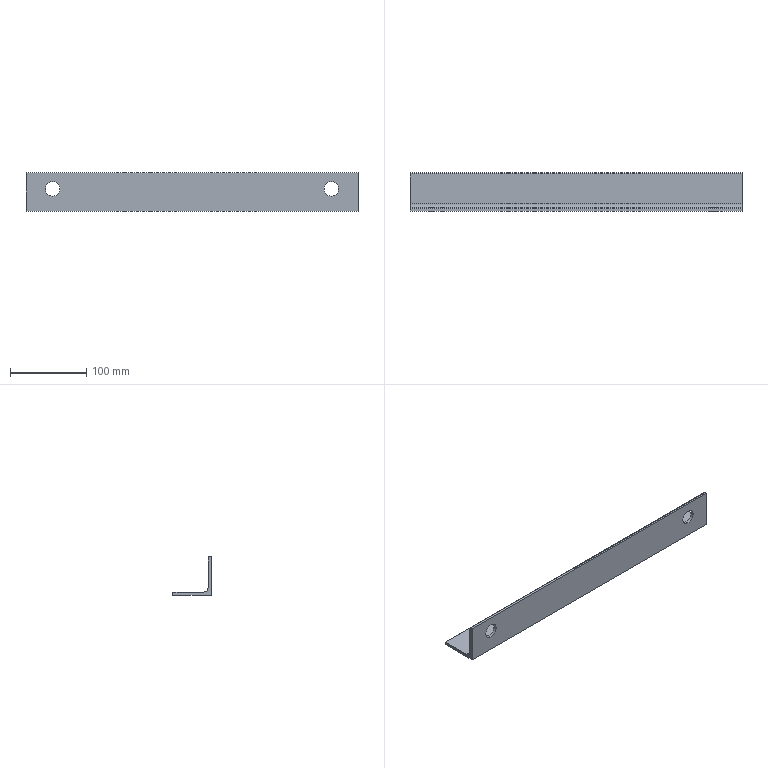Part | STEP file | 电柜楼梯角钢_Default<As Machined> | 1 solid | 15 faces | box 435 x 50 x 50 mm | volume 167265 mm3 | plane 8 | cylinder 7 | commonest cylinder face diameters 19 x4 2.66 x2 11 x1
STEP:
#1=CARTESIAN_POINT('',(0.,0.,0.));
#2=DIRECTION('',(0.,0.,1.));
#3=DIRECTION('',(1.,0.,0.));
#4=AXIS2_PLACEMENT_3D('',#1,#2,#3);
#5=CARTESIAN_POINT('',(-182.5,0.,38.585));
#6=VERTEX_POINT('',#5);
#7=CARTESIAN_POINT('',(-182.5,4.,38.585));
#8=VERTEX_POINT('',#7);
#9=CARTESIAN_POINT('',(-182.5,-6.,38.585));
#10=DIRECTION('',(0.,1.,0.));
#11=VECTOR('',#10,1.);
#12=LINE('',#9,#11);
#13=CARTESIAN_POINT('',(-182.5,-6.,29.085));
#14=DIRECTION('',(0.,1.,0.));
#15=DIRECTION('',(0.,0.,1.));
#16=AXIS2_PLACEMENT_3D('',#13,#14,#15);
#17=CYLINDRICAL_SURFACE('',#16,9.5);
#18=CARTESIAN_POINT('',(6.283,0.));
#19=DIRECTION('',(0.,1.));
#20=VECTOR('',#19,1.);
#21=LINE('',#18,#20);
#22=(GEOMETRIC_REPRESENTATION_CONTEXT(2)PARAMETRIC_REPRESENTATION_CONTEXT()REPRESENTATION_CONTEXT('',''));
#23=DEFINITIONAL_REPRESENTATION('',(#21),#22);
#24=PCURVE('',#17,#23);
#25=CARTESIAN_POINT('',(-182.5,-6.,29.085));
#26=DIRECTION('',(0.,1.,0.));
#27=DIRECTION('',(0.,0.,1.));
#28=AXIS2_PLACEMENT_3D('',#25,#26,#27);
#29=CYLINDRICAL_SURFACE('',#28,9.5);
#30=CARTESIAN_POINT('',(0.,0.));
#31=DIRECTION('',(0.,1.));
#32=VECTOR('',#31,1.);
#33=LINE('',#30,#32);
#34=(GEOMETRIC_REPRESENTATION_CONTEXT(2)PARAMETRIC_REPRESENTATION_CONTEXT()REPRESENTATION_CONTEXT('',''));
#35=DEFINITIONAL_REPRESENTATION('',(#33),#34);
#36=PCURVE('',#29,#35);
#37=SURFACE_CURVE('',#12,(#24,#36),.PCURVE_S1.);
#38=EDGE_CURVE('',#6,#8,#37,.T.);
#39=ORIENTED_EDGE('',*,*,#38,.T.);
#40=CARTESIAN_POINT('',(-182.5,4.,19.585));
#41=VERTEX_POINT('',#40);
#42=CARTESIAN_POINT('',(-182.5,4.,29.085));
#43=DIRECTION('',(0.,1.,0.));
#44=DIRECTION('',(0.,0.,1.));
#45=AXIS2_PLACEMENT_3D('',#42,#43,#44);
#46=CIRCLE('',#45,9.5);
#47=CARTESIAN_POINT('',(0.,10.));
#48=DIRECTION('',(1.,0.));
#49=VECTOR('',#48,1.);
#50=LINE('',#47,#49);
#51=(GEOMETRIC_REPRESENTATION_CONTEXT(2)PARAMETRIC_REPRESENTATION_CONTEXT()REPRESENTATION_CONTEXT('',''));
#52=DEFINITIONAL_REPRESENTATION('',(#50),#51);
#53=PCURVE('',#17,#52);
#54=CARTESIAN_POINT('',(217.5,4.,48.67));
#55=DIRECTION('',(0.,-1.,0.));
#56=DIRECTION('',(1.,0.,0.));
#57=AXIS2_PLACEMENT_3D('',#54,#55,#56);
#58=PLANE('',#57);
#59=CARTESIAN_POINT('',(-400.,-10.085));
#60=CARTESIAN_POINT('',(-383.546,-10.085));
#61=CARTESIAN_POINT('',(-391.773,-24.335));
#62=CARTESIAN_POINT('',(-400.,-38.585));
#63=CARTESIAN_POINT('',(-408.227,-24.335));
#64=CARTESIAN_POINT('',(-416.454,-10.085));
#65=CARTESIAN_POINT('',(-400.,-10.085));
#66=(BOUNDED_CURVE()B_SPLINE_CURVE(2,(#59,#60,#61,#62,#63,#64,#65),.UNSPECIFIED.,.T.,.F.)B_SPLINE_CURVE_WITH_KNOTS((1,2,2,2,2,1),(-2.094,0.,2.094,4.189,6.283,8.378),.UNSPECIFIED.)CURVE()GEOMETRIC_REPRESENTATION_ITEM()RATIONAL_B_SPLINE_CURVE((1.,0.5,1.,0.5,1.,0.5,1.))REPRESENTATION_ITEM(''));
#67=(GEOMETRIC_REPRESENTATION_CONTEXT(2)PARAMETRIC_REPRESENTATION_CONTEXT()REPRESENTATION_CONTEXT('',''));
#68=DEFINITIONAL_REPRESENTATION('',(#66),#67);
#69=PCURVE('',#58,#68);
#70=SURFACE_CURVE('',#46,(#53,#69),.PCURVE_S1.);
#71=EDGE_CURVE('',#41,#8,#70,.T.);
#72=ORIENTED_EDGE('',*,*,#71,.F.);
#73=CARTESIAN_POINT('',(-182.5,0.,19.585));
#74=VERTEX_POINT('',#73);
#75=CARTESIAN_POINT('',(-182.5,-6.,19.585));
#76=DIRECTION('',(0.,1.,0.));
#77=VECTOR('',#76,1.);
#78=LINE('',#75,#77);
#79=CARTESIAN_POINT('',(3.142,0.));
#80=DIRECTION('',(0.,1.));
#81=VECTOR('',#80,1.);
#82=LINE('',#79,#81);
#83=(GEOMETRIC_REPRESENTATION_CONTEXT(2)PARAMETRIC_REPRESENTATION_CONTEXT()REPRESENTATION_CONTEXT('',''));
#84=DEFINITIONAL_REPRESENTATION('',(#82),#83);
#85=PCURVE('',#17,#84);
#86=CARTESIAN_POINT('',(3.142,0.));
#87=DIRECTION('',(0.,1.));
#88=VECTOR('',#87,1.);
#89=LINE('',#86,#88);
#90=(GEOMETRIC_REPRESENTATION_CONTEXT(2)PARAMETRIC_REPRESENTATION_CONTEXT()REPRESENTATION_CONTEXT('',''));
#91=DEFINITIONAL_REPRESENTATION('',(#89),#90);
#92=PCURVE('',#29,#91);
#93=SURFACE_CURVE('',#78,(#85,#92),.PCURVE_S1.);
#94=EDGE_CURVE('',#74,#41,#93,.T.);
#95=ORIENTED_EDGE('',*,*,#94,.F.);
#96=CARTESIAN_POINT('',(-182.5,0.,29.085));
#97=DIRECTION('',(0.,1.,0.));
#98=DIRECTION('',(-1.,0.,0.));
#99=AXIS2_PLACEMENT_3D('',#96,#97,#98);
#100=CIRCLE('',#99,9.5);
#101=CARTESIAN_POINT('',(-1.571,6.));
#102=DIRECTION('',(1.,0.));
#103=VECTOR('',#102,1.);
#104=LINE('',#101,#103);
#105=(GEOMETRIC_REPRESENTATION_CONTEXT(2)PARAMETRIC_REPRESENTATION_CONTEXT()REPRESENTATION_CONTEXT('',''));
#106=DEFINITIONAL_REPRESENTATION('',(#104),#105);
#107=PCURVE('',#17,#106);
#108=CARTESIAN_POINT('',(217.5,0.,50.));
#109=DIRECTION('',(0.,1.,0.));
#110=DIRECTION('',(-1.,0.,0.));
#111=AXIS2_PLACEMENT_3D('',#108,#109,#110);
#112=PLANE('',#111);
#113=CARTESIAN_POINT('',(400.,-20.915));
#114=DIRECTION('',(1.,0.));
#115=AXIS2_PLACEMENT_2D('',#113,#114);
#116=CIRCLE('',#115,9.5);
#117=(GEOMETRIC_REPRESENTATION_CONTEXT(2)PARAMETRIC_REPRESENTATION_CONTEXT()REPRESENTATION_CONTEXT('',''));
#118=DEFINITIONAL_REPRESENTATION('',(#116),#117);
#119=PCURVE('',#112,#118);
#120=SURFACE_CURVE('',#100,(#107,#119),.PCURVE_S1.);
#121=EDGE_CURVE('',#74,#6,#120,.T.);
#122=ORIENTED_EDGE('',*,*,#121,.T.);
#123=EDGE_LOOP('',(#39,#72,#95,#122));
#124=FACE_BOUND('',#123,.F.);
#125=ADVANCED_FACE('',(#124),#17,.F.);
#126=CARTESIAN_POINT('',(182.5,0.,38.585));
#127=VERTEX_POINT('',#126);
#128=CARTESIAN_POINT('',(182.5,4.,38.585));
#129=VERTEX_POINT('',#128);
#130=CARTESIAN_POINT('',(182.5,-6.,38.585));
#131=DIRECTION('',(0.,1.,0.));
#132=VECTOR('',#131,1.);
#133=LINE('',#130,#132);
#134=CARTESIAN_POINT('',(182.5,-6.,29.085));
#135=DIRECTION('',(0.,1.,0.));
#136=DIRECTION('',(0.,0.,1.));
#137=AXIS2_PLACEMENT_3D('',#134,#135,#136);
#138=CYLINDRICAL_SURFACE('',#137,9.5);
#139=CARTESIAN_POINT('',(6.283,0.));
#140=DIRECTION('',(0.,1.));
#141=VECTOR('',#140,1.);
#142=LINE('',#139,#141);
#143=(GEOMETRIC_REPRESENTATION_CONTEXT(2)PARAMETRIC_REPRESENTATION_CONTEXT()REPRESENTATION_CONTEXT('',''));
#144=DEFINITIONAL_REPRESENTATION('',(#142),#143);
#145=PCURVE('',#138,#144);
#146=CARTESIAN_POINT('',(182.5,-6.,29.085));
#147=DIRECTION('',(0.,1.,0.));
#148=DIRECTION('',(0.,0.,1.));
#149=AXIS2_PLACEMENT_3D('',#146,#147,#148);
#150=CYLINDRICAL_SURFACE('',#149,9.5);
#151=CARTESIAN_POINT('',(0.,0.));
#152=DIRECTION('',(0.,1.));
#153=VECTOR('',#152,1.);
#154=LINE('',#151,#153);
#155=(GEOMETRIC_REPRESENTATION_CONTEXT(2)PARAMETRIC_REPRESENTATION_CONTEXT()REPRESENTATION_CONTEXT('',''));
#156=DEFINITIONAL_REPRESENTATION('',(#154),#155);
#157=PCURVE('',#150,#156);
#158=SURFACE_CURVE('',#133,(#145,#157),.PCURVE_S1.);
#159=EDGE_CURVE('',#127,#129,#158,.T.);
#160=ORIENTED_EDGE('',*,*,#159,.T.);
#161=CARTESIAN_POINT('',(182.5,4.,19.585));
#162=VERTEX_POINT('',#161);
#163=CARTESIAN_POINT('',(182.5,4.,29.085));
#164=DIRECTION('',(0.,1.,0.));
#165=DIRECTION('',(0.,0.,-1.));
#166=AXIS2_PLACEMENT_3D('',#163,#164,#165);
#167=CIRCLE('',#166,9.5);
#168=CARTESIAN_POINT('',(3.142,10.));
#169=DIRECTION('',(1.,0.));
#170=VECTOR('',#169,1.);
#171=LINE('',#168,#170);
#172=(GEOMETRIC_REPRESENTATION_CONTEXT(2)PARAMETRIC_REPRESENTATION_CONTEXT()REPRESENTATION_CONTEXT('',''));
#173=DEFINITIONAL_REPRESENTATION('',(#171),#172);
#174=PCURVE('',#138,#173);
#175=CARTESIAN_POINT('',(-35.,-29.085));
#176=CARTESIAN_POINT('',(-51.454,-29.085));
#177=CARTESIAN_POINT('',(-43.227,-14.835));
#178=CARTESIAN_POINT('',(-35.,-0.585));
#179=CARTESIAN_POINT('',(-26.773,-14.835));
#180=CARTESIAN_POINT('',(-18.546,-29.085));
#181=CARTESIAN_POINT('',(-35.,-29.085));
#182=(BOUNDED_CURVE()B_SPLINE_CURVE(2,(#175,#176,#177,#178,#179,#180,#181),.UNSPECIFIED.,.T.,.F.)B_SPLINE_CURVE_WITH_KNOTS((1,2,2,2,2,1),(-2.094,0.,2.094,4.189,6.283,8.378),.UNSPECIFIED.)CURVE()GEOMETRIC_REPRESENTATION_ITEM()RATIONAL_B_SPLINE_CURVE((1.,0.5,1.,0.5,1.,0.5,1.))REPRESENTATION_ITEM(''));
#183=(GEOMETRIC_REPRESENTATION_CONTEXT(2)PARAMETRIC_REPRESENTATION_CONTEXT()REPRESENTATION_CONTEXT('',''));
#184=DEFINITIONAL_REPRESENTATION('',(#182),#183);
#185=PCURVE('',#58,#184);
#186=SURFACE_CURVE('',#167,(#174,#185),.PCURVE_S1.);
#187=EDGE_CURVE('',#162,#129,#186,.T.);
#188=ORIENTED_EDGE('',*,*,#187,.F.);
#189=CARTESIAN_POINT('',(182.5,0.,19.585));
#190=VERTEX_POINT('',#189);
#191=CARTESIAN_POINT('',(182.5,-6.,19.585));
#192=DIRECTION('',(0.,1.,0.));
#193=VECTOR('',#192,1.);
#194=LINE('',#191,#193);
#195=CARTESIAN_POINT('',(3.142,0.));
#196=DIRECTION('',(0.,1.));
#197=VECTOR('',#196,1.);
#198=LINE('',#195,#197);
#199=(GEOMETRIC_REPRESENTATION_CONTEXT(2)PARAMETRIC_REPRESENTATION_CONTEXT()REPRESENTATION_CONTEXT('',''));
#200=DEFINITIONAL_REPRESENTATION('',(#198),#199);
#201=PCURVE('',#138,#200);
#202=CARTESIAN_POINT('',(3.142,0.));
#203=DIRECTION('',(0.,1.));
#204=VECTOR('',#203,1.);
#205=LINE('',#202,#204);
#206=(GEOMETRIC_REPRESENTATION_CONTEXT(2)PARAMETRIC_REPRESENTATION_CONTEXT()REPRESENTATION_CONTEXT('',''));
#207=DEFINITIONAL_REPRESENTATION('',(#205),#206);
#208=PCURVE('',#150,#207);
#209=SURFACE_CURVE('',#194,(#201,#208),.PCURVE_S1.);
#210=EDGE_CURVE('',#190,#162,#209,.T.);
#211=ORIENTED_EDGE('',*,*,#210,.F.);
#212=CARTESIAN_POINT('',(182.5,0.,29.085));
#213=DIRECTION('',(0.,1.,0.));
#214=DIRECTION('',(-1.,0.,0.));
#215=AXIS2_PLACEMENT_3D('',#212,#213,#214);
#216=CIRCLE('',#215,9.5);
#217=CARTESIAN_POINT('',(-1.571,6.));
#218=DIRECTION('',(1.,0.));
#219=VECTOR('',#218,1.);
#220=LINE('',#217,#219);
#221=(GEOMETRIC_REPRESENTATION_CONTEXT(2)PARAMETRIC_REPRESENTATION_CONTEXT()REPRESENTATION_CONTEXT('',''));
#222=DEFINITIONAL_REPRESENTATION('',(#220),#221);
#223=PCURVE('',#138,#222);
#224=CARTESIAN_POINT('',(35.,-20.915));
#225=DIRECTION('',(1.,0.));
#226=AXIS2_PLACEMENT_2D('',#224,#225);
#227=CIRCLE('',#226,9.5);
#228=(GEOMETRIC_REPRESENTATION_CONTEXT(2)PARAMETRIC_REPRESENTATION_CONTEXT()REPRESENTATION_CONTEXT('',''));
#229=DEFINITIONAL_REPRESENTATION('',(#227),#228);
#230=PCURVE('',#112,#229);
#231=SURFACE_CURVE('',#216,(#223,#230),.PCURVE_S1.);
#232=EDGE_CURVE('',#190,#127,#231,.T.);
#233=ORIENTED_EDGE('',*,*,#232,.T.);
#234=EDGE_LOOP('',(#160,#188,#211,#233));
#235=FACE_BOUND('',#234,.F.);
#236=ADVANCED_FACE('',(#235),#138,.F.);
#237=CARTESIAN_POINT('',(-217.5,50.,2.67));
#238=VERTEX_POINT('',#237);
#239=CARTESIAN_POINT('',(-217.5,48.67,4.));
#240=VERTEX_POINT('',#239);
#241=CARTESIAN_POINT('',(-217.5,48.67,2.67));
#242=DIRECTION('',(1.,0.,0.));
#243=DIRECTION('',(0.,1.,0.));
#244=AXIS2_PLACEMENT_3D('',#241,#242,#243);
#245=CIRCLE('',#244,1.33);
#246=CARTESIAN_POINT('',(217.5,48.67,2.67));
#247=DIRECTION('',(-1.,0.,0.));
#248=DIRECTION('',(0.,-1.,0.));
#249=AXIS2_PLACEMENT_3D('',#246,#247,#248);
#250=CYLINDRICAL_SURFACE('',#249,1.33);
#251=CARTESIAN_POINT('',(3.142,435.));
#252=DIRECTION('',(-1.,0.));
#253=VECTOR('',#252,1.);
#254=LINE('',#251,#253);
#255=(GEOMETRIC_REPRESENTATION_CONTEXT(2)PARAMETRIC_REPRESENTATION_CONTEXT()REPRESENTATION_CONTEXT('',''));
#256=DEFINITIONAL_REPRESENTATION('',(#254),#255);
#257=PCURVE('',#250,#256);
#258=CARTESIAN_POINT('',(-217.5,48.67,2.67));
#259=DIRECTION('',(1.,0.,0.));
#260=DIRECTION('',(0.,1.,0.));
#261=AXIS2_PLACEMENT_3D('',#258,#259,#260);
#262=PLANE('',#261);
#263=CARTESIAN_POINT('',(0.,0.));
#264=DIRECTION('',(1.,0.));
#265=AXIS2_PLACEMENT_2D('',#263,#264);
#266=CIRCLE('',#265,1.33);
#267=(GEOMETRIC_REPRESENTATION_CONTEXT(2)PARAMETRIC_REPRESENTATION_CONTEXT()REPRESENTATION_CONTEXT('',''));
#268=DEFINITIONAL_REPRESENTATION('',(#266),#267);
#269=PCURVE('',#262,#268);
#270=SURFACE_CURVE('',#245,(#257,#269),.PCURVE_S1.);
#271=EDGE_CURVE('',#238,#240,#270,.T.);
#272=ORIENTED_EDGE('',*,*,#271,.T.);
#273=CARTESIAN_POINT('',(217.5,48.67,4.));
#274=VERTEX_POINT('',#273);
#275=CARTESIAN_POINT('',(217.5,48.67,4.));
#276=DIRECTION('',(-1.,0.,0.));
#277=VECTOR('',#276,1.);
#278=LINE('',#275,#277);
#279=CARTESIAN_POINT('',(1.571,0.));
#280=DIRECTION('',(0.,1.));
#281=VECTOR('',#280,1.);
#282=LINE('',#279,#281);
#283=(GEOMETRIC_REPRESENTATION_CONTEXT(2)PARAMETRIC_REPRESENTATION_CONTEXT()REPRESENTATION_CONTEXT('',''));
#284=DEFINITIONAL_REPRESENTATION('',(#282),#283);
#285=PCURVE('',#250,#284);
#286=CARTESIAN_POINT('',(217.5,9.5,4.));
#287=DIRECTION('',(0.,0.,-1.));
#288=DIRECTION('',(-1.,0.,0.));
#289=AXIS2_PLACEMENT_3D('',#286,#287,#288);
#290=PLANE('',#289);
#291=CARTESIAN_POINT('',(0.,39.17));
#292=DIRECTION('',(1.,0.));
#293=VECTOR('',#292,1.);
#294=LINE('',#291,#293);
#295=(GEOMETRIC_REPRESENTATION_CONTEXT(2)PARAMETRIC_REPRESENTATION_CONTEXT()REPRESENTATION_CONTEXT('',''));
#296=DEFINITIONAL_REPRESENTATION('',(#294),#295);
#297=PCURVE('',#290,#296);
#298=SURFACE_CURVE('',#278,(#285,#297),.PCURVE_S1.);
#299=EDGE_CURVE('',#274,#240,#298,.T.);
#300=ORIENTED_EDGE('',*,*,#299,.F.);
#301=CARTESIAN_POINT('',(217.5,50.,2.67));
#302=VERTEX_POINT('',#301);
#303=CARTESIAN_POINT('',(217.5,48.67,2.67));
#304=DIRECTION('',(1.,0.,0.));
#305=DIRECTION('',(0.,1.,0.));
#306=AXIS2_PLACEMENT_3D('',#303,#304,#305);
#307=CIRCLE('',#306,1.33);
#308=CARTESIAN_POINT('',(3.142,0.));
#309=DIRECTION('',(-1.,0.));
#310=VECTOR('',#309,1.);
#311=LINE('',#308,#310);
#312=(GEOMETRIC_REPRESENTATION_CONTEXT(2)PARAMETRIC_REPRESENTATION_CONTEXT()REPRESENTATION_CONTEXT('',''));
#313=DEFINITIONAL_REPRESENTATION('',(#311),#312);
#314=PCURVE('',#250,#313);
#315=CARTESIAN_POINT('',(217.5,48.67,2.67));
#316=DIRECTION('',(1.,0.,0.));
#317=DIRECTION('',(0.,1.,0.));
#318=AXIS2_PLACEMENT_3D('',#315,#316,#317);
#319=PLANE('',#318);
#320=CARTESIAN_POINT('',(0.,0.));
#321=DIRECTION('',(1.,0.));
#322=AXIS2_PLACEMENT_2D('',#320,#321);
#323=CIRCLE('',#322,1.33);
#324=(GEOMETRIC_REPRESENTATION_CONTEXT(2)PARAMETRIC_REPRESENTATION_CONTEXT()REPRESENTATION_CONTEXT('',''));
#325=DEFINITIONAL_REPRESENTATION('',(#323),#324);
#326=PCURVE('',#319,#325);
#327=SURFACE_CURVE('',#307,(#314,#326),.PCURVE_S1.);
#328=EDGE_CURVE('',#302,#274,#327,.T.);
#329=ORIENTED_EDGE('',*,*,#328,.F.);
#330=CARTESIAN_POINT('',(217.5,50.,2.67));
#331=DIRECTION('',(-1.,0.,0.));
#332=VECTOR('',#331,1.);
#333=LINE('',#330,#332);
#334=CARTESIAN_POINT('',(3.142,0.));
#335=DIRECTION('',(0.,1.));
#336=VECTOR('',#335,1.);
#337=LINE('',#334,#336);
#338=(GEOMETRIC_REPRESENTATION_CONTEXT(2)PARAMETRIC_REPRESENTATION_CONTEXT()REPRESENTATION_CONTEXT('',''));
#339=DEFINITIONAL_REPRESENTATION('',(#337),#338);
#340=PCURVE('',#250,#339);
#341=CARTESIAN_POINT('',(217.5,50.,2.67));
#342=DIRECTION('',(0.,-1.,0.));
#343=DIRECTION('',(1.,0.,0.));
#344=AXIS2_PLACEMENT_3D('',#341,#342,#343);
#345=PLANE('',#344);
#346=CARTESIAN_POINT('',(0.,0.));
#347=DIRECTION('',(-1.,0.));
#348=VECTOR('',#347,1.);
#349=LINE('',#346,#348);
#350=(GEOMETRIC_REPRESENTATION_CONTEXT(2)PARAMETRIC_REPRESENTATION_CONTEXT()REPRESENTATION_CONTEXT('',''));
#351=DEFINITIONAL_REPRESENTATION('',(#349),#350);
#352=PCURVE('',#345,#351);
#353=SURFACE_CURVE('',#333,(#340,#352),.PCURVE_S1.);
#354=EDGE_CURVE('',#302,#238,#353,.T.);
#355=ORIENTED_EDGE('',*,*,#354,.T.);
#356=EDGE_LOOP('',(#272,#300,#329,#355));
#357=FACE_BOUND('',#356,.T.);
#358=ADVANCED_FACE('',(#357),#250,.T.);
#359=CARTESIAN_POINT('',(-217.5,9.5,4.));
#360=VERTEX_POINT('',#359);
#361=CARTESIAN_POINT('',(-217.5,9.5,4.));
#362=DIRECTION('',(0.,-1.,0.));
#363=VECTOR('',#362,1.);
#364=LINE('',#361,#363);
#365=CARTESIAN_POINT('',(435.,0.));
#366=DIRECTION('',(0.,-1.));
#367=VECTOR('',#366,1.);
#368=LINE('',#365,#367);
#369=(GEOMETRIC_REPRESENTATION_CONTEXT(2)PARAMETRIC_REPRESENTATION_CONTEXT()REPRESENTATION_CONTEXT('',''));
#370=DEFINITIONAL_REPRESENTATION('',(#368),#369);
#371=PCURVE('',#290,#370);
#372=CARTESIAN_POINT('',(-39.17,1.33));
#373=DIRECTION('',(-1.,0.));
#374=VECTOR('',#373,1.);
#375=LINE('',#372,#374);
#376=(GEOMETRIC_REPRESENTATION_CONTEXT(2)PARAMETRIC_REPRESENTATION_CONTEXT()REPRESENTATION_CONTEXT('',''));
#377=DEFINITIONAL_REPRESENTATION('',(#375),#376);
#378=PCURVE('',#262,#377);
#379=SURFACE_CURVE('',#364,(#371,#378),.PCURVE_S1.);
#380=EDGE_CURVE('',#240,#360,#379,.T.);
#381=ORIENTED_EDGE('',*,*,#380,.T.);
#382=CARTESIAN_POINT('',(217.5,9.5,4.));
#383=VERTEX_POINT('',#382);
#384=CARTESIAN_POINT('',(217.5,9.5,4.));
#385=DIRECTION('',(-1.,0.,0.));
#386=VECTOR('',#385,1.);
#387=LINE('',#384,#386);
#388=CARTESIAN_POINT('',(0.,0.));
#389=DIRECTION('',(1.,0.));
#390=VECTOR('',#389,1.);
#391=LINE('',#388,#390);
#392=(GEOMETRIC_REPRESENTATION_CONTEXT(2)PARAMETRIC_REPRESENTATION_CONTEXT()REPRESENTATION_CONTEXT('',''));
#393=DEFINITIONAL_REPRESENTATION('',(#391),#392);
#394=PCURVE('',#290,#393);
#395=CARTESIAN_POINT('',(217.5,9.5,9.5));
#396=DIRECTION('',(-1.,0.,0.));
#397=DIRECTION('',(0.,-1.,0.));
#398=AXIS2_PLACEMENT_3D('',#395,#396,#397);
#399=CYLINDRICAL_SURFACE('',#398,5.5);
#400=CARTESIAN_POINT('',(4.712,0.));
#401=DIRECTION('',(0.,1.));
#402=VECTOR('',#401,1.);
#403=LINE('',#400,#402);
#404=(GEOMETRIC_REPRESENTATION_CONTEXT(2)PARAMETRIC_REPRESENTATION_CONTEXT()REPRESENTATION_CONTEXT('',''));
#405=DEFINITIONAL_REPRESENTATION('',(#403),#404);
#406=PCURVE('',#399,#405);
#407=SURFACE_CURVE('',#387,(#394,#406),.PCURVE_S1.);
#408=EDGE_CURVE('',#383,#360,#407,.T.);
#409=ORIENTED_EDGE('',*,*,#408,.F.);
#410=CARTESIAN_POINT('',(217.5,9.5,4.));
#411=DIRECTION('',(0.,-1.,0.));
#412=VECTOR('',#411,1.);
#413=LINE('',#410,#412);
#414=CARTESIAN_POINT('',(0.,0.));
#415=DIRECTION('',(0.,-1.));
#416=VECTOR('',#415,1.);
#417=LINE('',#414,#416);
#418=(GEOMETRIC_REPRESENTATION_CONTEXT(2)PARAMETRIC_REPRESENTATION_CONTEXT()REPRESENTATION_CONTEXT('',''));
#419=DEFINITIONAL_REPRESENTATION('',(#417),#418);
#420=PCURVE('',#290,#419);
#421=CARTESIAN_POINT('',(-39.17,1.33));
#422=DIRECTION('',(-1.,0.));
#423=VECTOR('',#422,1.);
#424=LINE('',#421,#423);
#425=(GEOMETRIC_REPRESENTATION_CONTEXT(2)PARAMETRIC_REPRESENTATION_CONTEXT()REPRESENTATION_CONTEXT('',''));
#426=DEFINITIONAL_REPRESENTATION('',(#424),#425);
#427=PCURVE('',#319,#426);
#428=SURFACE_CURVE('',#413,(#420,#427),.PCURVE_S1.);
#429=EDGE_CURVE('',#274,#383,#428,.T.);
#430=ORIENTED_EDGE('',*,*,#429,.F.);
#431=ORIENTED_EDGE('',*,*,#299,.T.);
#432=EDGE_LOOP('',(#381,#409,#430,#431));
#433=FACE_BOUND('',#432,.T.);
#434=ADVANCED_FACE('',(#433),#290,.F.);
#435=ORIENTED_EDGE('',*,*,#408,.F.);
#436=CARTESIAN_POINT('',(217.5,4.,9.5));
#437=VERTEX_POINT('',#436);
#438=CARTESIAN_POINT('',(217.5,9.5,9.5));
#439=DIRECTION('',(-1.,0.,0.));
#440=DIRECTION('',(0.,1.,0.));
#441=AXIS2_PLACEMENT_3D('',#438,#439,#440);
#442=CIRCLE('',#441,5.5);
#443=CARTESIAN_POINT('',(3.142,0.));
#444=DIRECTION('',(1.,0.));
#445=VECTOR('',#444,1.);
#446=LINE('',#443,#445);
#447=(GEOMETRIC_REPRESENTATION_CONTEXT(2)PARAMETRIC_REPRESENTATION_CONTEXT()REPRESENTATION_CONTEXT('',''));
#448=DEFINITIONAL_REPRESENTATION('',(#446),#447);
#449=PCURVE('',#399,#448);
#450=CARTESIAN_POINT('',(-33.67,6.83));
#451=CARTESIAN_POINT('',(-33.67,-2.696));
#452=CARTESIAN_POINT('',(-41.92,2.067));
#453=CARTESIAN_POINT('',(-50.17,6.83));
#454=CARTESIAN_POINT('',(-41.92,11.593));
#455=CARTESIAN_POINT('',(-33.67,16.356));
#456=CARTESIAN_POINT('',(-33.67,6.83));
#457=(BOUNDED_CURVE()B_SPLINE_CURVE(2,(#450,#451,#452,#453,#454,#455,#456),.UNSPECIFIED.,.T.,.F.)B_SPLINE_CURVE_WITH_KNOTS((1,2,2,2,2,1),(-2.094,0.,2.094,4.189,6.283,8.378),.UNSPECIFIED.)CURVE()GEOMETRIC_REPRESENTATION_ITEM()RATIONAL_B_SPLINE_CURVE((1.,0.5,1.,0.5,1.,0.5,1.))REPRESENTATION_ITEM(''));
#458=(GEOMETRIC_REPRESENTATION_CONTEXT(2)PARAMETRIC_REPRESENTATION_CONTEXT()REPRESENTATION_CONTEXT('',''));
#459=DEFINITIONAL_REPRESENTATION('',(#457),#458);
#460=PCURVE('',#319,#459);
#461=SURFACE_CURVE('',#442,(#449,#460),.PCURVE_S1.);
#462=EDGE_CURVE('',#383,#437,#461,.T.);
#463=ORIENTED_EDGE('',*,*,#462,.T.);
#464=CARTESIAN_POINT('',(-217.5,4.,9.5));
#465=VERTEX_POINT('',#464);
#466=CARTESIAN_POINT('',(217.5,4.,9.5));
#467=DIRECTION('',(-1.,0.,0.));
#468=VECTOR('',#467,1.);
#469=LINE('',#466,#468);
#470=CARTESIAN_POINT('',(6.283,0.));
#471=DIRECTION('',(0.,1.));
#472=VECTOR('',#471,1.);
#473=LINE('',#470,#472);
#474=(GEOMETRIC_REPRESENTATION_CONTEXT(2)PARAMETRIC_REPRESENTATION_CONTEXT()REPRESENTATION_CONTEXT('',''));
#475=DEFINITIONAL_REPRESENTATION('',(#473),#474);
#476=PCURVE('',#399,#475);
#477=CARTESIAN_POINT('',(0.,-39.17));
#478=DIRECTION('',(-1.,0.));
#479=VECTOR('',#478,1.);
#480=LINE('',#477,#479);
#481=(GEOMETRIC_REPRESENTATION_CONTEXT(2)PARAMETRIC_REPRESENTATION_CONTEXT()REPRESENTATION_CONTEXT('',''));
#482=DEFINITIONAL_REPRESENTATION('',(#480),#481);
#483=PCURVE('',#58,#482);
#484=SURFACE_CURVE('',#469,(#476,#483),.PCURVE_S1.);
#485=EDGE_CURVE('',#437,#465,#484,.T.);
#486=ORIENTED_EDGE('',*,*,#485,.T.);
#487=CARTESIAN_POINT('',(-217.5,9.5,9.5));
#488=DIRECTION('',(-1.,0.,0.));
#489=DIRECTION('',(0.,1.,0.));
#490=AXIS2_PLACEMENT_3D('',#487,#488,#489);
#491=CIRCLE('',#490,5.5);
#492=CARTESIAN_POINT('',(3.142,435.));
#493=DIRECTION('',(1.,0.));
#494=VECTOR('',#493,1.);
#495=LINE('',#492,#494);
#496=(GEOMETRIC_REPRESENTATION_CONTEXT(2)PARAMETRIC_REPRESENTATION_CONTEXT()REPRESENTATION_CONTEXT('',''));
#497=DEFINITIONAL_REPRESENTATION('',(#495),#496);
#498=PCURVE('',#399,#497);
#499=CARTESIAN_POINT('',(-33.67,6.83));
#500=CARTESIAN_POINT('',(-33.67,-2.696));
#501=CARTESIAN_POINT('',(-41.92,2.067));
#502=CARTESIAN_POINT('',(-50.17,6.83));
#503=CARTESIAN_POINT('',(-41.92,11.593));
#504=CARTESIAN_POINT('',(-33.67,16.356));
#505=CARTESIAN_POINT('',(-33.67,6.83));
#506=(BOUNDED_CURVE()B_SPLINE_CURVE(2,(#499,#500,#501,#502,#503,#504,#505),.UNSPECIFIED.,.T.,.F.)B_SPLINE_CURVE_WITH_KNOTS((1,2,2,2,2,1),(-2.094,0.,2.094,4.189,6.283,8.378),.UNSPECIFIED.)CURVE()GEOMETRIC_REPRESENTATION_ITEM()RATIONAL_B_SPLINE_CURVE((1.,0.5,1.,0.5,1.,0.5,1.))REPRESENTATION_ITEM(''));
#507=(GEOMETRIC_REPRESENTATION_CONTEXT(2)PARAMETRIC_REPRESENTATION_CONTEXT()REPRESENTATION_CONTEXT('',''));
#508=DEFINITIONAL_REPRESENTATION('',(#506),#507);
#509=PCURVE('',#262,#508);
#510=SURFACE_CURVE('',#491,(#498,#509),.PCURVE_S1.);
#511=EDGE_CURVE('',#360,#465,#510,.T.);
#512=ORIENTED_EDGE('',*,*,#511,.F.);
#513=EDGE_LOOP('',(#435,#463,#486,#512));
#514=FACE_BOUND('',#513,.F.);
#515=ADVANCED_FACE('',(#514),#399,.F.);
#516=CARTESIAN_POINT('',(-182.5,4.,29.085));
#517=DIRECTION('',(0.,1.,0.));
#518=DIRECTION('',(0.,0.,1.));
#519=AXIS2_PLACEMENT_3D('',#516,#517,#518);
#520=CIRCLE('',#519,9.5);
#521=CARTESIAN_POINT('',(-400.,-10.085));
#522=CARTESIAN_POINT('',(-383.546,-10.085));
#523=CARTESIAN_POINT('',(-391.773,-24.335));
#524=CARTESIAN_POINT('',(-400.,-38.585));
#525=CARTESIAN_POINT('',(-408.227,-24.335));
#526=CARTESIAN_POINT('',(-416.454,-10.085));
#527=CARTESIAN_POINT('',(-400.,-10.085));
#528=(BOUNDED_CURVE()B_SPLINE_CURVE(2,(#521,#522,#523,#524,#525,#526,#527),.UNSPECIFIED.,.T.,.F.)B_SPLINE_CURVE_WITH_KNOTS((1,2,2,2,2,1),(-2.094,0.,2.094,4.189,6.283,8.378),.UNSPECIFIED.)CURVE()GEOMETRIC_REPRESENTATION_ITEM()RATIONAL_B_SPLINE_CURVE((1.,0.5,1.,0.5,1.,0.5,1.))REPRESENTATION_ITEM(''));
#529=(GEOMETRIC_REPRESENTATION_CONTEXT(2)PARAMETRIC_REPRESENTATION_CONTEXT()REPRESENTATION_CONTEXT('',''));
#530=DEFINITIONAL_REPRESENTATION('',(#528),#529);
#531=PCURVE('',#58,#530);
#532=CARTESIAN_POINT('',(0.,10.));
#533=DIRECTION('',(1.,0.));
#534=VECTOR('',#533,1.);
#535=LINE('',#532,#534);
#536=(GEOMETRIC_REPRESENTATION_CONTEXT(2)PARAMETRIC_REPRESENTATION_CONTEXT()REPRESENTATION_CONTEXT('',''));
#537=DEFINITIONAL_REPRESENTATION('',(#535),#536);
#538=PCURVE('',#29,#537);
#539=SURFACE_CURVE('',#520,(#531,#538),.PCURVE_S1.);
#540=EDGE_CURVE('',#8,#41,#539,.T.);
#541=ORIENTED_EDGE('',*,*,#540,.F.);
#542=ORIENTED_EDGE('',*,*,#71,.F.);
#543=EDGE_LOOP('',(#541,#542));
#544=FACE_BOUND('',#543,.T.);
#545=CARTESIAN_POINT('',(182.5,4.,29.085));
#546=DIRECTION('',(0.,1.,0.));
#547=DIRECTION('',(0.,0.,-1.));
#548=AXIS2_PLACEMENT_3D('',#545,#546,#547);
#549=CIRCLE('',#548,9.5);
#550=CARTESIAN_POINT('',(-35.,-29.085));
#551=CARTESIAN_POINT('',(-51.454,-29.085));
#552=CARTESIAN_POINT('',(-43.227,-14.835));
#553=CARTESIAN_POINT('',(-35.,-0.585));
#554=CARTESIAN_POINT('',(-26.773,-14.835));
#555=CARTESIAN_POINT('',(-18.546,-29.085));
#556=CARTESIAN_POINT('',(-35.,-29.085));
#557=(BOUNDED_CURVE()B_SPLINE_CURVE(2,(#550,#551,#552,#553,#554,#555,#556),.UNSPECIFIED.,.T.,.F.)B_SPLINE_CURVE_WITH_KNOTS((1,2,2,2,2,1),(-2.094,0.,2.094,4.189,6.283,8.378),.UNSPECIFIED.)CURVE()GEOMETRIC_REPRESENTATION_ITEM()RATIONAL_B_SPLINE_CURVE((1.,0.5,1.,0.5,1.,0.5,1.))REPRESENTATION_ITEM(''));
#558=(GEOMETRIC_REPRESENTATION_CONTEXT(2)PARAMETRIC_REPRESENTATION_CONTEXT()REPRESENTATION_CONTEXT('',''));
#559=DEFINITIONAL_REPRESENTATION('',(#557),#558);
#560=PCURVE('',#58,#559);
#561=CARTESIAN_POINT('',(-3.142,10.));
#562=DIRECTION('',(1.,0.));
#563=VECTOR('',#562,1.);
#564=LINE('',#561,#563);
#565=(GEOMETRIC_REPRESENTATION_CONTEXT(2)PARAMETRIC_REPRESENTATION_CONTEXT()REPRESENTATION_CONTEXT('',''));
#566=DEFINITIONAL_REPRESENTATION('',(#564),#565);
#567=PCURVE('',#150,#566);
#568=SURFACE_CURVE('',#549,(#560,#567),.PCURVE_S1.);
#569=EDGE_CURVE('',#129,#162,#568,.T.);
#570=ORIENTED_EDGE('',*,*,#569,.F.);
#571=ORIENTED_EDGE('',*,*,#187,.F.);
#572=EDGE_LOOP('',(#570,#571));
#573=FACE_BOUND('',#572,.T.);
#574=CARTESIAN_POINT('',(-217.5,4.,48.67));
#575=VERTEX_POINT('',#574);
#576=CARTESIAN_POINT('',(-217.5,4.,48.67));
#577=DIRECTION('',(0.,0.,1.));
#578=VECTOR('',#577,1.);
#579=LINE('',#576,#578);
#580=CARTESIAN_POINT('',(-435.,0.));
#581=DIRECTION('',(0.,1.));
#582=VECTOR('',#581,1.);
#583=LINE('',#580,#582);
#584=(GEOMETRIC_REPRESENTATION_CONTEXT(2)PARAMETRIC_REPRESENTATION_CONTEXT()REPRESENTATION_CONTEXT('',''));
#585=DEFINITIONAL_REPRESENTATION('',(#583),#584);
#586=PCURVE('',#58,#585);
#587=CARTESIAN_POINT('',(-44.67,46.));
#588=DIRECTION('',(0.,1.));
#589=VECTOR('',#588,1.);
#590=LINE('',#587,#589);
#591=(GEOMETRIC_REPRESENTATION_CONTEXT(2)PARAMETRIC_REPRESENTATION_CONTEXT()REPRESENTATION_CONTEXT('',''));
#592=DEFINITIONAL_REPRESENTATION('',(#590),#591);
#593=PCURVE('',#262,#592);
#594=SURFACE_CURVE('',#579,(#586,#593),.PCURVE_S1.);
#595=EDGE_CURVE('',#465,#575,#594,.T.);
#596=ORIENTED_EDGE('',*,*,#595,.T.);
#597=CARTESIAN_POINT('',(217.5,4.,48.67));
#598=VERTEX_POINT('',#597);
#599=CARTESIAN_POINT('',(217.5,4.,48.67));
#600=DIRECTION('',(-1.,0.,0.));
#601=VECTOR('',#600,1.);
#602=LINE('',#599,#601);
#603=CARTESIAN_POINT('',(0.,0.));
#604=DIRECTION('',(-1.,0.));
#605=VECTOR('',#604,1.);
#606=LINE('',#603,#605);
#607=(GEOMETRIC_REPRESENTATION_CONTEXT(2)PARAMETRIC_REPRESENTATION_CONTEXT()REPRESENTATION_CONTEXT('',''));
#608=DEFINITIONAL_REPRESENTATION('',(#606),#607);
#609=PCURVE('',#58,#608);
#610=CARTESIAN_POINT('',(217.5,2.67,48.67));
#611=DIRECTION('',(-1.,0.,0.));
#612=DIRECTION('',(0.,-1.,0.));
#613=AXIS2_PLACEMENT_3D('',#610,#611,#612);
#614=CYLINDRICAL_SURFACE('',#613,1.33);
#615=CARTESIAN_POINT('',(3.142,0.));
#616=DIRECTION('',(0.,1.));
#617=VECTOR('',#616,1.);
#618=LINE('',#615,#617);
#619=(GEOMETRIC_REPRESENTATION_CONTEXT(2)PARAMETRIC_REPRESENTATION_CONTEXT()REPRESENTATION_CONTEXT('',''));
#620=DEFINITIONAL_REPRESENTATION('',(#618),#619);
#621=PCURVE('',#614,#620);
#622=SURFACE_CURVE('',#602,(#609,#621),.PCURVE_S1.);
#623=EDGE_CURVE('',#598,#575,#622,.T.);
#624=ORIENTED_EDGE('',*,*,#623,.F.);
#625=CARTESIAN_POINT('',(217.5,4.,48.67));
#626=DIRECTION('',(0.,0.,1.));
#627=VECTOR('',#626,1.);
#628=LINE('',#625,#627);
#629=CARTESIAN_POINT('',(0.,0.));
#630=DIRECTION('',(0.,1.));
#631=VECTOR('',#630,1.);
#632=LINE('',#629,#631);
#633=(GEOMETRIC_REPRESENTATION_CONTEXT(2)PARAMETRIC_REPRESENTATION_CONTEXT()REPRESENTATION_CONTEXT('',''));
#634=DEFINITIONAL_REPRESENTATION('',(#632),#633);
#635=PCURVE('',#58,#634);
#636=CARTESIAN_POINT('',(-44.67,46.));
#637=DIRECTION('',(0.,1.));
#638=VECTOR('',#637,1.);
#639=LINE('',#636,#638);
#640=(GEOMETRIC_REPRESENTATION_CONTEXT(2)PARAMETRIC_REPRESENTATION_CONTEXT()REPRESENTATION_CONTEXT('',''));
#641=DEFINITIONAL_REPRESENTATION('',(#639),#640);
#642=PCURVE('',#319,#641);
#643=SURFACE_CURVE('',#628,(#635,#642),.PCURVE_S1.);
#644=EDGE_CURVE('',#437,#598,#643,.T.);
#645=ORIENTED_EDGE('',*,*,#644,.F.);
#646=ORIENTED_EDGE('',*,*,#485,.T.);
#647=EDGE_LOOP('',(#596,#624,#645,#646));
#648=FACE_BOUND('',#647,.T.);
#649=ADVANCED_FACE('',(#544,#573,#648),#58,.F.);
#650=CARTESIAN_POINT('',(-217.5,2.67,50.));
#651=VERTEX_POINT('',#650);
#652=CARTESIAN_POINT('',(-217.5,2.67,48.67));
#653=DIRECTION('',(1.,0.,0.));
#654=DIRECTION('',(0.,1.,0.));
#655=AXIS2_PLACEMENT_3D('',#652,#653,#654);
#656=CIRCLE('',#655,1.33);
#657=CARTESIAN_POINT('',(3.142,435.));
#658=DIRECTION('',(-1.,0.));
#659=VECTOR('',#658,1.);
#660=LINE('',#657,#659);
#661=(GEOMETRIC_REPRESENTATION_CONTEXT(2)PARAMETRIC_REPRESENTATION_CONTEXT()REPRESENTATION_CONTEXT('',''));
#662=DEFINITIONAL_REPRESENTATION('',(#660),#661);
#663=PCURVE('',#614,#662);
#664=CARTESIAN_POINT('',(-46.,46.));
#665=DIRECTION('',(1.,0.));
#666=AXIS2_PLACEMENT_2D('',#664,#665);
#667=CIRCLE('',#666,1.33);
#668=(GEOMETRIC_REPRESENTATION_CONTEXT(2)PARAMETRIC_REPRESENTATION_CONTEXT()REPRESENTATION_CONTEXT('',''));
#669=DEFINITIONAL_REPRESENTATION('',(#667),#668);
#670=PCURVE('',#262,#669);
#671=SURFACE_CURVE('',#656,(#663,#670),.PCURVE_S1.);
#672=EDGE_CURVE('',#575,#651,#671,.T.);
#673=ORIENTED_EDGE('',*,*,#672,.T.);
#674=CARTESIAN_POINT('',(217.5,2.67,50.));
#675=VERTEX_POINT('',#674);
#676=CARTESIAN_POINT('',(217.5,2.67,50.));
#677=DIRECTION('',(-1.,0.,0.));
#678=VECTOR('',#677,1.);
#679=LINE('',#676,#678);
#680=CARTESIAN_POINT('',(1.571,0.));
#681=DIRECTION('',(0.,1.));
#682=VECTOR('',#681,1.);
#683=LINE('',#680,#682);
#684=(GEOMETRIC_REPRESENTATION_CONTEXT(2)PARAMETRIC_REPRESENTATION_CONTEXT()REPRESENTATION_CONTEXT('',''));
#685=DEFINITIONAL_REPRESENTATION('',(#683),#684);
#686=PCURVE('',#614,#685);
#687=CARTESIAN_POINT('',(217.5,0.,50.));
#688=DIRECTION('',(0.,0.,-1.));
#689=DIRECTION('',(0.,1.,0.));
#690=AXIS2_PLACEMENT_3D('',#687,#688,#689);
#691=PLANE('',#690);
#692=CARTESIAN_POINT('',(2.67,0.));
#693=DIRECTION('',(0.,-1.));
#694=VECTOR('',#693,1.);
#695=LINE('',#692,#694);
#696=(GEOMETRIC_REPRESENTATION_CONTEXT(2)PARAMETRIC_REPRESENTATION_CONTEXT()REPRESENTATION_CONTEXT('',''));
#697=DEFINITIONAL_REPRESENTATION('',(#695),#696);
#698=PCURVE('',#691,#697);
#699=SURFACE_CURVE('',#679,(#686,#698),.PCURVE_S1.);
#700=EDGE_CURVE('',#675,#651,#699,.T.);
#701=ORIENTED_EDGE('',*,*,#700,.F.);
#702=CARTESIAN_POINT('',(217.5,2.67,48.67));
#703=DIRECTION('',(1.,0.,0.));
#704=DIRECTION('',(0.,1.,0.));
#705=AXIS2_PLACEMENT_3D('',#702,#703,#704);
#706=CIRCLE('',#705,1.33);
#707=CARTESIAN_POINT('',(3.142,0.));
#708=DIRECTION('',(-1.,0.));
#709=VECTOR('',#708,1.);
#710=LINE('',#707,#709);
#711=(GEOMETRIC_REPRESENTATION_CONTEXT(2)PARAMETRIC_REPRESENTATION_CONTEXT()REPRESENTATION_CONTEXT('',''));
#712=DEFINITIONAL_REPRESENTATION('',(#710),#711);
#713=PCURVE('',#614,#712);
#714=CARTESIAN_POINT('',(-46.,46.));
#715=DIRECTION('',(1.,0.));
#716=AXIS2_PLACEMENT_2D('',#714,#715);
#717=CIRCLE('',#716,1.33);
#718=(GEOMETRIC_REPRESENTATION_CONTEXT(2)PARAMETRIC_REPRESENTATION_CONTEXT()REPRESENTATION_CONTEXT('',''));
#719=DEFINITIONAL_REPRESENTATION('',(#717),#718);
#720=PCURVE('',#319,#719);
#721=SURFACE_CURVE('',#706,(#713,#720),.PCURVE_S1.);
#722=EDGE_CURVE('',#598,#675,#721,.T.);
#723=ORIENTED_EDGE('',*,*,#722,.F.);
#724=ORIENTED_EDGE('',*,*,#623,.T.);
#725=EDGE_LOOP('',(#673,#701,#723,#724));
#726=FACE_BOUND('',#725,.T.);
#727=ADVANCED_FACE('',(#726),#614,.T.);
#728=CARTESIAN_POINT('',(-217.5,0.,50.));
#729=VERTEX_POINT('',#728);
#730=CARTESIAN_POINT('',(-217.5,0.,50.));
#731=DIRECTION('',(0.,-1.,0.));
#732=VECTOR('',#731,1.);
#733=LINE('',#730,#732);
#734=CARTESIAN_POINT('',(0.,-435.));
#735=DIRECTION('',(-1.,0.));
#736=VECTOR('',#735,1.);
#737=LINE('',#734,#736);
#738=(GEOMETRIC_REPRESENTATION_CONTEXT(2)PARAMETRIC_REPRESENTATION_CONTEXT()REPRESENTATION_CONTEXT('',''));
#739=DEFINITIONAL_REPRESENTATION('',(#737),#738);
#740=PCURVE('',#691,#739);
#741=CARTESIAN_POINT('',(-48.67,47.33));
#742=DIRECTION('',(-1.,0.));
#743=VECTOR('',#742,1.);
#744=LINE('',#741,#743);
#745=(GEOMETRIC_REPRESENTATION_CONTEXT(2)PARAMETRIC_REPRESENTATION_CONTEXT()REPRESENTATION_CONTEXT('',''));
#746=DEFINITIONAL_REPRESENTATION('',(#744),#745);
#747=PCURVE('',#262,#746);
#748=SURFACE_CURVE('',#733,(#740,#747),.PCURVE_S1.);
#749=EDGE_CURVE('',#651,#729,#748,.T.);
#750=ORIENTED_EDGE('',*,*,#749,.T.);
#751=CARTESIAN_POINT('',(217.5,0.,50.));
#752=VERTEX_POINT('',#751);
#753=CARTESIAN_POINT('',(217.5,0.,50.));
#754=DIRECTION('',(-1.,0.,0.));
#755=VECTOR('',#754,1.);
#756=LINE('',#753,#755);
#757=CARTESIAN_POINT('',(0.,0.));
#758=DIRECTION('',(0.,-1.));
#759=VECTOR('',#758,1.);
#760=LINE('',#757,#759);
#761=(GEOMETRIC_REPRESENTATION_CONTEXT(2)PARAMETRIC_REPRESENTATION_CONTEXT()REPRESENTATION_CONTEXT('',''));
#762=DEFINITIONAL_REPRESENTATION('',(#760),#761);
#763=PCURVE('',#691,#762);
#764=CARTESIAN_POINT('',(0.,0.));
#765=DIRECTION('',(1.,0.));
#766=VECTOR('',#765,1.);
#767=LINE('',#764,#766);
#768=(GEOMETRIC_REPRESENTATION_CONTEXT(2)PARAMETRIC_REPRESENTATION_CONTEXT()REPRESENTATION_CONTEXT('',''));
#769=DEFINITIONAL_REPRESENTATION('',(#767),#768);
#770=PCURVE('',#112,#769);
#771=SURFACE_CURVE('',#756,(#763,#770),.PCURVE_S1.);
#772=EDGE_CURVE('',#752,#729,#771,.T.);
#773=ORIENTED_EDGE('',*,*,#772,.F.);
#774=CARTESIAN_POINT('',(217.5,0.,50.));
#775=DIRECTION('',(0.,-1.,0.));
#776=VECTOR('',#775,1.);
#777=LINE('',#774,#776);
#778=CARTESIAN_POINT('',(0.,0.));
#779=DIRECTION('',(-1.,0.));
#780=VECTOR('',#779,1.);
#781=LINE('',#778,#780);
#782=(GEOMETRIC_REPRESENTATION_CONTEXT(2)PARAMETRIC_REPRESENTATION_CONTEXT()REPRESENTATION_CONTEXT('',''));
#783=DEFINITIONAL_REPRESENTATION('',(#781),#782);
#784=PCURVE('',#691,#783);
#785=CARTESIAN_POINT('',(-48.67,47.33));
#786=DIRECTION('',(-1.,0.));
#787=VECTOR('',#786,1.);
#788=LINE('',#785,#787);
#789=(GEOMETRIC_REPRESENTATION_CONTEXT(2)PARAMETRIC_REPRESENTATION_CONTEXT()REPRESENTATION_CONTEXT('',''));
#790=DEFINITIONAL_REPRESENTATION('',(#788),#789);
#791=PCURVE('',#319,#790);
#792=SURFACE_CURVE('',#777,(#784,#791),.PCURVE_S1.);
#793=EDGE_CURVE('',#675,#752,#792,.T.);
#794=ORIENTED_EDGE('',*,*,#793,.F.);
#795=ORIENTED_EDGE('',*,*,#700,.T.);
#796=EDGE_LOOP('',(#750,#773,#794,#795));
#797=FACE_BOUND('',#796,.T.);
#798=ADVANCED_FACE('',(#797),#691,.F.);
#799=CARTESIAN_POINT('',(-182.5,0.,29.085));
#800=DIRECTION('',(0.,1.,0.));
#801=DIRECTION('',(-1.,0.,0.));
#802=AXIS2_PLACEMENT_3D('',#799,#800,#801);
#803=CIRCLE('',#802,9.5);
#804=CARTESIAN_POINT('',(400.,-20.915));
#805=DIRECTION('',(1.,0.));
#806=AXIS2_PLACEMENT_2D('',#804,#805);
#807=CIRCLE('',#806,9.5);
#808=(GEOMETRIC_REPRESENTATION_CONTEXT(2)PARAMETRIC_REPRESENTATION_CONTEXT()REPRESENTATION_CONTEXT('',''));
#809=DEFINITIONAL_REPRESENTATION('',(#807),#808);
#810=PCURVE('',#112,#809);
#811=CARTESIAN_POINT('',(-1.571,6.));
#812=DIRECTION('',(1.,0.));
#813=VECTOR('',#812,1.);
#814=LINE('',#811,#813);
#815=(GEOMETRIC_REPRESENTATION_CONTEXT(2)PARAMETRIC_REPRESENTATION_CONTEXT()REPRESENTATION_CONTEXT('',''));
#816=DEFINITIONAL_REPRESENTATION('',(#814),#815);
#817=PCURVE('',#29,#816);
#818=SURFACE_CURVE('',#803,(#810,#817),.PCURVE_S1.);
#819=EDGE_CURVE('',#6,#74,#818,.T.);
#820=ORIENTED_EDGE('',*,*,#819,.T.);
#821=ORIENTED_EDGE('',*,*,#121,.T.);
#822=EDGE_LOOP('',(#820,#821));
#823=FACE_BOUND('',#822,.T.);
#824=CARTESIAN_POINT('',(182.5,0.,29.085));
#825=DIRECTION('',(0.,1.,0.));
#826=DIRECTION('',(-1.,0.,0.));
#827=AXIS2_PLACEMENT_3D('',#824,#825,#826);
#828=CIRCLE('',#827,9.5);
#829=CARTESIAN_POINT('',(35.,-20.915));
#830=DIRECTION('',(1.,0.));
#831=AXIS2_PLACEMENT_2D('',#829,#830);
#832=CIRCLE('',#831,9.5);
#833=(GEOMETRIC_REPRESENTATION_CONTEXT(2)PARAMETRIC_REPRESENTATION_CONTEXT()REPRESENTATION_CONTEXT('',''));
#834=DEFINITIONAL_REPRESENTATION('',(#832),#833);
#835=PCURVE('',#112,#834);
#836=CARTESIAN_POINT('',(-1.571,6.));
#837=DIRECTION('',(1.,0.));
#838=VECTOR('',#837,1.);
#839=LINE('',#836,#838);
#840=(GEOMETRIC_REPRESENTATION_CONTEXT(2)PARAMETRIC_REPRESENTATION_CONTEXT()REPRESENTATION_CONTEXT('',''));
#841=DEFINITIONAL_REPRESENTATION('',(#839),#840);
#842=PCURVE('',#150,#841);
#843=SURFACE_CURVE('',#828,(#835,#842),.PCURVE_S1.);
#844=EDGE_CURVE('',#127,#190,#843,.T.);
#845=ORIENTED_EDGE('',*,*,#844,.T.);
#846=ORIENTED_EDGE('',*,*,#232,.T.);
#847=EDGE_LOOP('',(#845,#846));
#848=FACE_BOUND('',#847,.T.);
#849=CARTESIAN_POINT('',(-217.5,0.,0.));
#850=VERTEX_POINT('',#849);
#851=CARTESIAN_POINT('',(-217.5,0.,50.));
#852=DIRECTION('',(0.,0.,-1.));
#853=VECTOR('',#852,1.);
#854=LINE('',#851,#853);
#855=CARTESIAN_POINT('',(435.,0.));
#856=DIRECTION('',(0.,-1.));
#857=VECTOR('',#856,1.);
#858=LINE('',#855,#857);
#859=(GEOMETRIC_REPRESENTATION_CONTEXT(2)PARAMETRIC_REPRESENTATION_CONTEXT()REPRESENTATION_CONTEXT('',''));
#860=DEFINITIONAL_REPRESENTATION('',(#858),#859);
#861=PCURVE('',#112,#860);
#862=CARTESIAN_POINT('',(-48.67,47.33));
#863=DIRECTION('',(0.,-1.));
#864=VECTOR('',#863,1.);
#865=LINE('',#862,#864);
#866=(GEOMETRIC_REPRESENTATION_CONTEXT(2)PARAMETRIC_REPRESENTATION_CONTEXT()REPRESENTATION_CONTEXT('',''));
#867=DEFINITIONAL_REPRESENTATION('',(#865),#866);
#868=PCURVE('',#262,#867);
#869=SURFACE_CURVE('',#854,(#861,#868),.PCURVE_S1.);
#870=EDGE_CURVE('',#729,#850,#869,.T.);
#871=ORIENTED_EDGE('',*,*,#870,.T.);
#872=CARTESIAN_POINT('',(217.5,0.,0.));
#873=VERTEX_POINT('',#872);
#874=CARTESIAN_POINT('',(217.5,0.,0.));
#875=DIRECTION('',(-1.,0.,0.));
#876=VECTOR('',#875,1.);
#877=LINE('',#874,#876);
#878=CARTESIAN_POINT('',(0.,-50.));
#879=DIRECTION('',(1.,0.));
#880=VECTOR('',#879,1.);
#881=LINE('',#878,#880);
#882=(GEOMETRIC_REPRESENTATION_CONTEXT(2)PARAMETRIC_REPRESENTATION_CONTEXT()REPRESENTATION_CONTEXT('',''));
#883=DEFINITIONAL_REPRESENTATION('',(#881),#882);
#884=PCURVE('',#112,#883);
#885=CARTESIAN_POINT('',(217.5,0.,0.));
#886=DIRECTION('',(0.,0.,1.));
#887=DIRECTION('',(1.,0.,0.));
#888=AXIS2_PLACEMENT_3D('',#885,#886,#887);
#889=PLANE('',#888);
#890=CARTESIAN_POINT('',(0.,0.));
#891=DIRECTION('',(-1.,0.));
#892=VECTOR('',#891,1.);
#893=LINE('',#890,#892);
#894=(GEOMETRIC_REPRESENTATION_CONTEXT(2)PARAMETRIC_REPRESENTATION_CONTEXT()REPRESENTATION_CONTEXT('',''));
#895=DEFINITIONAL_REPRESENTATION('',(#893),#894);
#896=PCURVE('',#889,#895);
#897=SURFACE_CURVE('',#877,(#884,#896),.PCURVE_S1.);
#898=EDGE_CURVE('',#873,#850,#897,.T.);
#899=ORIENTED_EDGE('',*,*,#898,.F.);
#900=CARTESIAN_POINT('',(217.5,0.,50.));
#901=DIRECTION('',(0.,0.,-1.));
#902=VECTOR('',#901,1.);
#903=LINE('',#900,#902);
#904=CARTESIAN_POINT('',(0.,0.));
#905=DIRECTION('',(0.,-1.));
#906=VECTOR('',#905,1.);
#907=LINE('',#904,#906);
#908=(GEOMETRIC_REPRESENTATION_CONTEXT(2)PARAMETRIC_REPRESENTATION_CONTEXT()REPRESENTATION_CONTEXT('',''));
#909=DEFINITIONAL_REPRESENTATION('',(#907),#908);
#910=PCURVE('',#112,#909);
#911=CARTESIAN_POINT('',(-48.67,47.33));
#912=DIRECTION('',(0.,-1.));
#913=VECTOR('',#912,1.);
#914=LINE('',#911,#913);
#915=(GEOMETRIC_REPRESENTATION_CONTEXT(2)PARAMETRIC_REPRESENTATION_CONTEXT()REPRESENTATION_CONTEXT('',''));
#916=DEFINITIONAL_REPRESENTATION('',(#914),#915);
#917=PCURVE('',#319,#916);
#918=SURFACE_CURVE('',#903,(#910,#917),.PCURVE_S1.);
#919=EDGE_CURVE('',#752,#873,#918,.T.);
#920=ORIENTED_EDGE('',*,*,#919,.F.);
#921=ORIENTED_EDGE('',*,*,#772,.T.);
#922=EDGE_LOOP('',(#871,#899,#920,#921));
#923=FACE_BOUND('',#922,.T.);
#924=ADVANCED_FACE('',(#823,#848,#923),#112,.F.);
#925=CARTESIAN_POINT('',(-217.5,50.,0.));
#926=VERTEX_POINT('',#925);
#927=CARTESIAN_POINT('',(-217.5,0.,0.));
#928=DIRECTION('',(0.,1.,0.));
#929=VECTOR('',#928,1.);
#930=LINE('',#927,#929);
#931=CARTESIAN_POINT('',(-435.,0.));
#932=DIRECTION('',(0.,1.));
#933=VECTOR('',#932,1.);
#934=LINE('',#931,#933);
#935=(GEOMETRIC_REPRESENTATION_CONTEXT(2)PARAMETRIC_REPRESENTATION_CONTEXT()REPRESENTATION_CONTEXT('',''));
#936=DEFINITIONAL_REPRESENTATION('',(#934),#935);
#937=PCURVE('',#889,#936);
#938=CARTESIAN_POINT('',(-48.67,-2.67));
#939=DIRECTION('',(1.,0.));
#940=VECTOR('',#939,1.);
#941=LINE('',#938,#940);
#942=(GEOMETRIC_REPRESENTATION_CONTEXT(2)PARAMETRIC_REPRESENTATION_CONTEXT()REPRESENTATION_CONTEXT('',''));
#943=DEFINITIONAL_REPRESENTATION('',(#941),#942);
#944=PCURVE('',#262,#943);
#945=SURFACE_CURVE('',#930,(#937,#944),.PCURVE_S1.);
#946=EDGE_CURVE('',#850,#926,#945,.T.);
#947=ORIENTED_EDGE('',*,*,#946,.T.);
#948=CARTESIAN_POINT('',(217.5,50.,0.));
#949=VERTEX_POINT('',#948);
#950=CARTESIAN_POINT('',(217.5,50.,0.));
#951=DIRECTION('',(-1.,0.,0.));
#952=VECTOR('',#951,1.);
#953=LINE('',#950,#952);
#954=CARTESIAN_POINT('',(0.,50.));
#955=DIRECTION('',(-1.,0.));
#956=VECTOR('',#955,1.);
#957=LINE('',#954,#956);
#958=(GEOMETRIC_REPRESENTATION_CONTEXT(2)PARAMETRIC_REPRESENTATION_CONTEXT()REPRESENTATION_CONTEXT('',''));
#959=DEFINITIONAL_REPRESENTATION('',(#957),#958);
#960=PCURVE('',#889,#959);
#961=CARTESIAN_POINT('',(0.,-2.67));
#962=DIRECTION('',(-1.,0.));
#963=VECTOR('',#962,1.);
#964=LINE('',#961,#963);
#965=(GEOMETRIC_REPRESENTATION_CONTEXT(2)PARAMETRIC_REPRESENTATION_CONTEXT()REPRESENTATION_CONTEXT('',''));
#966=DEFINITIONAL_REPRESENTATION('',(#964),#965);
#967=PCURVE('',#345,#966);
#968=SURFACE_CURVE('',#953,(#960,#967),.PCURVE_S1.);
#969=EDGE_CURVE('',#949,#926,#968,.T.);
#970=ORIENTED_EDGE('',*,*,#969,.F.);
#971=CARTESIAN_POINT('',(217.5,0.,0.));
#972=DIRECTION('',(0.,1.,0.));
#973=VECTOR('',#972,1.);
#974=LINE('',#971,#973);
#975=CARTESIAN_POINT('',(0.,0.));
#976=DIRECTION('',(0.,1.));
#977=VECTOR('',#976,1.);
#978=LINE('',#975,#977);
#979=(GEOMETRIC_REPRESENTATION_CONTEXT(2)PARAMETRIC_REPRESENTATION_CONTEXT()REPRESENTATION_CONTEXT('',''));
#980=DEFINITIONAL_REPRESENTATION('',(#978),#979);
#981=PCURVE('',#889,#980);
#982=CARTESIAN_POINT('',(-48.67,-2.67));
#983=DIRECTION('',(1.,0.));
#984=VECTOR('',#983,1.);
#985=LINE('',#982,#984);
#986=(GEOMETRIC_REPRESENTATION_CONTEXT(2)PARAMETRIC_REPRESENTATION_CONTEXT()REPRESENTATION_CONTEXT('',''));
#987=DEFINITIONAL_REPRESENTATION('',(#985),#986);
#988=PCURVE('',#319,#987);
#989=SURFACE_CURVE('',#974,(#981,#988),.PCURVE_S1.);
#990=EDGE_CURVE('',#873,#949,#989,.T.);
#991=ORIENTED_EDGE('',*,*,#990,.F.);
#992=ORIENTED_EDGE('',*,*,#898,.T.);
#993=EDGE_LOOP('',(#947,#970,#991,#992));
#994=FACE_BOUND('',#993,.T.);
#995=ADVANCED_FACE('',(#994),#889,.F.);
#996=CARTESIAN_POINT('',(-217.5,50.,2.67));
#997=DIRECTION('',(0.,0.,1.));
#998=VECTOR('',#997,1.);
#999=LINE('',#996,#998);
#1000=CARTESIAN_POINT('',(-435.,0.));
#1001=DIRECTION('',(0.,1.));
#1002=VECTOR('',#1001,1.);
#1003=LINE('',#1000,#1002);
#1004=(GEOMETRIC_REPRESENTATION_CONTEXT(2)PARAMETRIC_REPRESENTATION_CONTEXT()REPRESENTATION_CONTEXT('',''));
#1005=DEFINITIONAL_REPRESENTATION('',(#1003),#1004);
#1006=PCURVE('',#345,#1005);
#1007=CARTESIAN_POINT('',(1.33,0.));
#1008=DIRECTION('',(0.,1.));
#1009=VECTOR('',#1008,1.);
#1010=LINE('',#1007,#1009);
#1011=(GEOMETRIC_REPRESENTATION_CONTEXT(2)PARAMETRIC_REPRESENTATION_CONTEXT()REPRESENTATION_CONTEXT('',''));
#1012=DEFINITIONAL_REPRESENTATION('',(#1010),#1011);
#1013=PCURVE('',#262,#1012);
#1014=SURFACE_CURVE('',#999,(#1006,#1013),.PCURVE_S1.);
#1015=EDGE_CURVE('',#926,#238,#1014,.T.);
#1016=ORIENTED_EDGE('',*,*,#1015,.T.);
#1017=ORIENTED_EDGE('',*,*,#354,.F.);
#1018=CARTESIAN_POINT('',(217.5,50.,2.67));
#1019=DIRECTION('',(0.,0.,1.));
#1020=VECTOR('',#1019,1.);
#1021=LINE('',#1018,#1020);
#1022=CARTESIAN_POINT('',(0.,0.));
#1023=DIRECTION('',(0.,1.));
#1024=VECTOR('',#1023,1.);
#1025=LINE('',#1022,#1024);
#1026=(GEOMETRIC_REPRESENTATION_CONTEXT(2)PARAMETRIC_REPRESENTATION_CONTEXT()REPRESENTATION_CONTEXT('',''));
#1027=DEFINITIONAL_REPRESENTATION('',(#1025),#1026);
#1028=PCURVE('',#345,#1027);
#1029=CARTESIAN_POINT('',(1.33,0.));
#1030=DIRECTION('',(0.,1.));
#1031=VECTOR('',#1030,1.);
#1032=LINE('',#1029,#1031);
#1033=(GEOMETRIC_REPRESENTATION_CONTEXT(2)PARAMETRIC_REPRESENTATION_CONTEXT()REPRESENTATION_CONTEXT('',''));
#1034=DEFINITIONAL_REPRESENTATION('',(#1032),#1033);
#1035=PCURVE('',#319,#1034);
#1036=SURFACE_CURVE('',#1021,(#1028,#1035),.PCURVE_S1.);
#1037=EDGE_CURVE('',#949,#302,#1036,.T.);
#1038=ORIENTED_EDGE('',*,*,#1037,.F.);
#1039=ORIENTED_EDGE('',*,*,#969,.T.);
#1040=EDGE_LOOP('',(#1016,#1017,#1038,#1039));
#1041=FACE_BOUND('',#1040,.T.);
#1042=ADVANCED_FACE('',(#1041),#345,.F.);
#1043=ORIENTED_EDGE('',*,*,#328,.T.);
#1044=ORIENTED_EDGE('',*,*,#429,.T.);
#1045=ORIENTED_EDGE('',*,*,#462,.T.);
#1046=ORIENTED_EDGE('',*,*,#644,.T.);
#1047=ORIENTED_EDGE('',*,*,#722,.T.);
#1048=ORIENTED_EDGE('',*,*,#793,.T.);
#1049=ORIENTED_EDGE('',*,*,#919,.T.);
#1050=ORIENTED_EDGE('',*,*,#990,.T.);
#1051=ORIENTED_EDGE('',*,*,#1037,.T.);
#1052=EDGE_LOOP('',(#1043,#1044,#1045,#1046,#1047,#1048,#1049,#1050,#1051));
#1053=FACE_BOUND('',#1052,.T.);
#1054=ADVANCED_FACE('',(#1053),#319,.T.);
#1055=ORIENTED_EDGE('',*,*,#271,.F.);
#1056=ORIENTED_EDGE('',*,*,#1015,.F.);
#1057=ORIENTED_EDGE('',*,*,#946,.F.);
#1058=ORIENTED_EDGE('',*,*,#870,.F.);
#1059=ORIENTED_EDGE('',*,*,#749,.F.);
#1060=ORIENTED_EDGE('',*,*,#672,.F.);
#1061=ORIENTED_EDGE('',*,*,#595,.F.);
#1062=ORIENTED_EDGE('',*,*,#511,.F.);
#1063=ORIENTED_EDGE('',*,*,#380,.F.);
#1064=EDGE_LOOP('',(#1055,#1056,#1057,#1058,#1059,#1060,#1061,#1062,#1063));
#1065=FACE_BOUND('',#1064,.T.);
#1066=ADVANCED_FACE('',(#1065),#262,.F.);
#1067=ORIENTED_EDGE('',*,*,#569,.F.);
#1068=ORIENTED_EDGE('',*,*,#159,.F.);
#1069=ORIENTED_EDGE('',*,*,#844,.T.);
#1070=ORIENTED_EDGE('',*,*,#210,.T.);
#1071=EDGE_LOOP('',(#1067,#1068,#1069,#1070));
#1072=FACE_BOUND('',#1071,.F.);
#1073=ADVANCED_FACE('',(#1072),#150,.F.);
#1074=ORIENTED_EDGE('',*,*,#540,.F.);
#1075=ORIENTED_EDGE('',*,*,#38,.F.);
#1076=ORIENTED_EDGE('',*,*,#819,.T.);
#1077=ORIENTED_EDGE('',*,*,#94,.T.);
#1078=EDGE_LOOP('',(#1074,#1075,#1076,#1077));
#1079=FACE_BOUND('',#1078,.F.);
#1080=ADVANCED_FACE('',(#1079),#29,.F.);
#1081=CLOSED_SHELL('',(#125,#236,#358,#434,#515,#649,#727,#798,#924,#995,#1042,#1054,#1066,#1073,#1080));
#1082=MANIFOLD_SOLID_BREP('',#1081);
#1083=(LENGTH_UNIT()NAMED_UNIT(*)SI_UNIT(.MILLI.,.METRE.));
#1084=UNCERTAINTY_MEASURE_WITH_UNIT(LENGTH_MEASURE(0.0000001),#1083,'','');
#1085=(NAMED_UNIT(*)PLANE_ANGLE_UNIT()SI_UNIT($,.RADIAN.));
#1086=(NAMED_UNIT(*)SI_UNIT($,.STERADIAN.)SOLID_ANGLE_UNIT());
#1087=(GEOMETRIC_REPRESENTATION_CONTEXT(3)GLOBAL_UNCERTAINTY_ASSIGNED_CONTEXT((#1084))GLOBAL_UNIT_ASSIGNED_CONTEXT((#1083,#1085,#1086))REPRESENTATION_CONTEXT('',''));
#1088=ADVANCED_BREP_SHAPE_REPRESENTATION('',(#4,#1082),#1087);